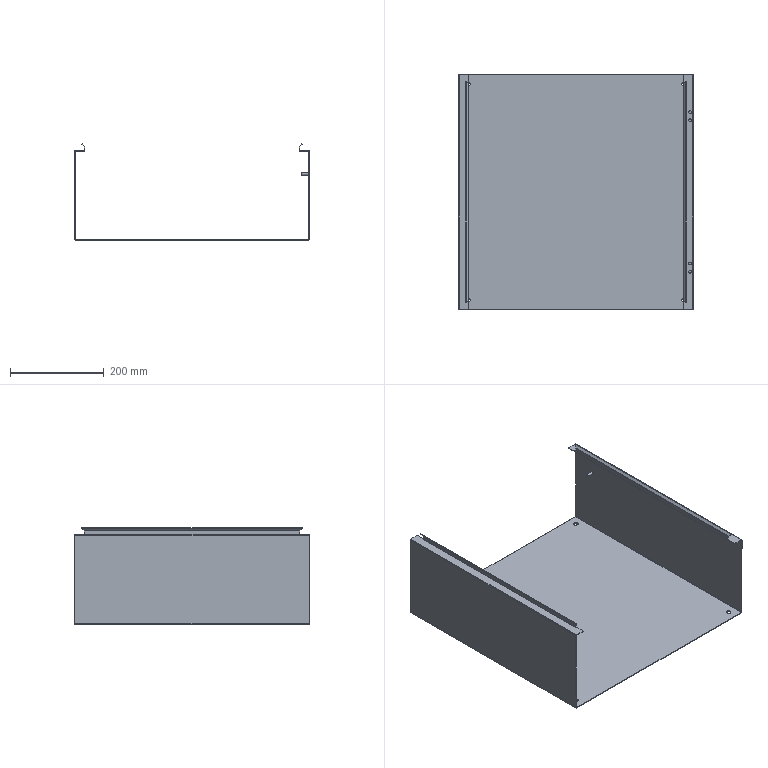Part | SolidWorks | features EdgeFlange 6, LPattern 4, ICE 3, SMBaseFlange 3, FlatPattern 1, SheetMetal 1 | 1 solid | 109 faces | box 500 x 500 x 205.157 mm | volume 710210 mm3 | plane 75 | cylinder 34 | commonest cylinder face diameters 6 x10 0.2 x8 3.2 x8 9 x8